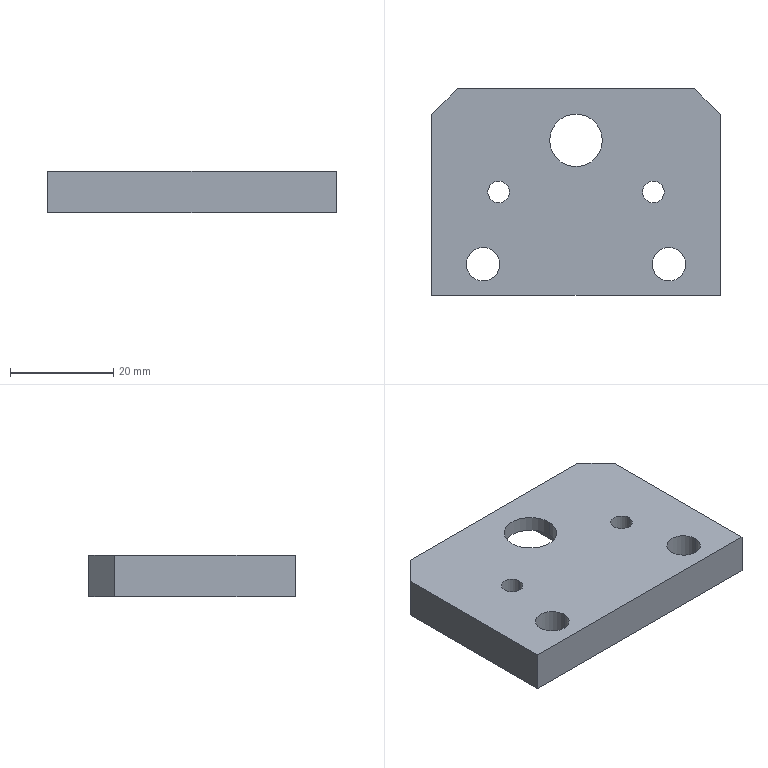Part | STEP file | BU-B05a | 1 solid | 24 faces | box 56 x 40 x 8 mm | volume 14978 mm3 | cylinder 12 | plane 12 | commonest cylinder face diameters 4.2 x4 6.5 x4 5 x2 10.2 x2